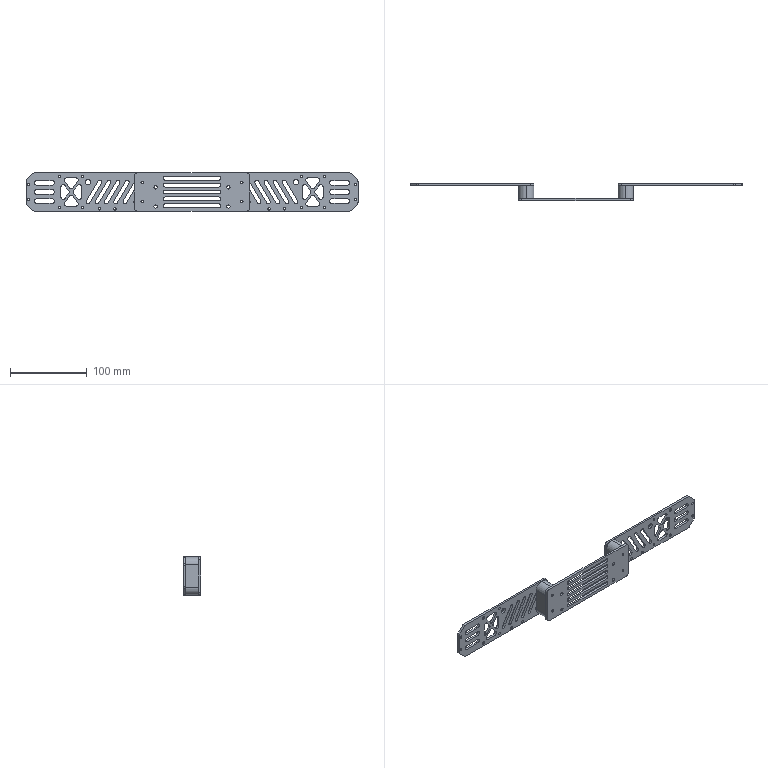Part | SolidWorks | features ICE 8, Fillet 7, Chamfer 1, Extrusion 1 | 5 solids | 274 faces | box 433.1 x 23 x 50 mm | volume 82463 mm3 | cylinder 178 | plane 96 | commonest cylinder face diameters 3.2 x56 6 x50 5 x40 4.2 x8 7 x8 8 x8